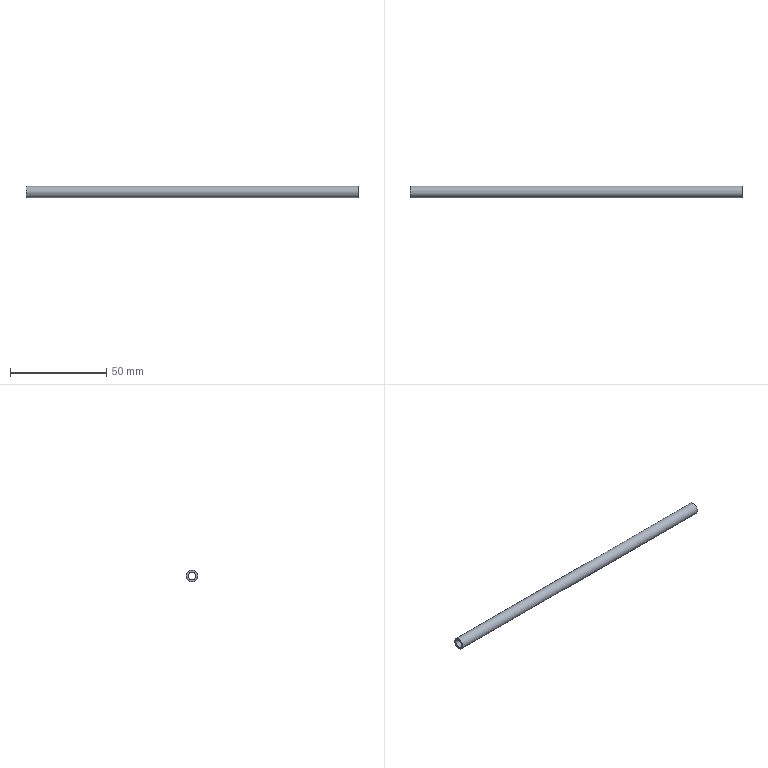Part | NX | features solid 2 | 1 solid | 4 faces | box 172.875 x 6 x 6 mm | volume 2716 mm3 | cylinder 2 | plane 2 | commonest cylinder face diameters 4 x1 6 x1
STEP:
#1=CARTESIAN_POINT('',(460.,-45.,347.));
#2=VERTEX_POINT('',#1);
#3=CARTESIAN_POINT('',(460.,-43.,347.));
#4=DIRECTION('',(-1.,0.,0.));
#5=DIRECTION('',(0.,-1.,0.));
#6=AXIS2_PLACEMENT_3D('',#3,#4,#5);
#7=CIRCLE('',#6,2.);
#8=EDGE_CURVE('',#2,#2,#7,.T.);
#9=ORIENTED_EDGE('',*,*,#8,.F.);
#10=EDGE_LOOP('',(#9));
#11=FACE_BOUND('',#10,.T.);
#12=CARTESIAN_POINT('',(287.125,-45.,347.));
#13=VERTEX_POINT('',#12);
#14=CARTESIAN_POINT('',(287.125,-43.,347.));
#15=DIRECTION('',(-1.,0.,0.));
#16=DIRECTION('',(0.,-1.,0.));
#17=AXIS2_PLACEMENT_3D('',#14,#15,#16);
#18=CIRCLE('',#17,2.);
#19=EDGE_CURVE('',#13,#13,#18,.T.);
#20=ORIENTED_EDGE('',*,*,#19,.T.);
#21=EDGE_LOOP('',(#20));
#22=FACE_BOUND('',#21,.T.);
#23=CARTESIAN_POINT('',(166.176,-43.,347.));
#24=DIRECTION('',(1.,0.,0.));
#25=DIRECTION('',(0.,1.,0.));
#26=AXIS2_PLACEMENT_3D('',#23,#24,#25);
#27=CYLINDRICAL_SURFACE('',#26,2.);
#28=ADVANCED_FACE('',(#11,#22),#27,.F.);
#29=CARTESIAN_POINT('',(460.,-46.,347.));
#30=VERTEX_POINT('',#29);
#31=CARTESIAN_POINT('',(460.,-43.,347.));
#32=DIRECTION('',(-1.,0.,0.));
#33=DIRECTION('',(0.,-1.,0.));
#34=AXIS2_PLACEMENT_3D('',#31,#32,#33);
#35=CIRCLE('',#34,3.);
#36=EDGE_CURVE('',#30,#30,#35,.T.);
#37=ORIENTED_EDGE('',*,*,#36,.T.);
#38=EDGE_LOOP('',(#37));
#39=FACE_BOUND('',#38,.T.);
#40=CARTESIAN_POINT('',(287.125,-46.,347.));
#41=VERTEX_POINT('',#40);
#42=CARTESIAN_POINT('',(287.125,-43.,347.));
#43=DIRECTION('',(-1.,0.,0.));
#44=DIRECTION('',(0.,-1.,0.));
#45=AXIS2_PLACEMENT_3D('',#42,#43,#44);
#46=CIRCLE('',#45,3.);
#47=EDGE_CURVE('',#41,#41,#46,.T.);
#48=ORIENTED_EDGE('',*,*,#47,.F.);
#49=EDGE_LOOP('',(#48));
#50=FACE_BOUND('',#49,.T.);
#51=CARTESIAN_POINT('',(166.176,-43.,347.));
#52=DIRECTION('',(1.,0.,0.));
#53=DIRECTION('',(0.,1.,0.));
#54=AXIS2_PLACEMENT_3D('',#51,#52,#53);
#55=CYLINDRICAL_SURFACE('',#54,3.);
#56=ADVANCED_FACE('',(#39,#50),#55,.T.);
#57=ORIENTED_EDGE('',*,*,#8,.T.);
#58=EDGE_LOOP('',(#57));
#59=FACE_BOUND('',#58,.T.);
#60=ORIENTED_EDGE('',*,*,#36,.F.);
#61=EDGE_LOOP('',(#60));
#62=FACE_BOUND('',#61,.T.);
#63=CARTESIAN_POINT('',(460.,-43.,347.));
#64=DIRECTION('',(-1.,0.,0.));
#65=DIRECTION('',(0.,-1.,0.));
#66=AXIS2_PLACEMENT_3D('',#63,#64,#65);
#67=PLANE('',#66);
#68=ADVANCED_FACE('',(#59,#62),#67,.F.);
#69=ORIENTED_EDGE('',*,*,#19,.F.);
#70=EDGE_LOOP('',(#69));
#71=FACE_BOUND('',#70,.T.);
#72=ORIENTED_EDGE('',*,*,#47,.T.);
#73=EDGE_LOOP('',(#72));
#74=FACE_BOUND('',#73,.T.);
#75=CARTESIAN_POINT('',(287.125,87.83,185.));
#76=DIRECTION('',(-1.,0.,0.));
#77=DIRECTION('',(0.,-1.,0.));
#78=AXIS2_PLACEMENT_3D('',#75,#76,#77);
#79=PLANE('',#78);
#80=ADVANCED_FACE('',(#71,#74),#79,.T.);
#81=CLOSED_SHELL('',(#28,#56,#68,#80));
#82=MANIFOLD_SOLID_BREP('',#81);
#83=(LENGTH_UNIT()NAMED_UNIT(*)SI_UNIT(.MILLI.,.METRE.));
#84=UNCERTAINTY_MEASURE_WITH_UNIT(LENGTH_MEASURE(0.00001),#83,'','');
#85=(NAMED_UNIT(*)PLANE_ANGLE_UNIT()SI_UNIT($,.RADIAN.));
#86=(NAMED_UNIT(*)SI_UNIT($,.STERADIAN.)SOLID_ANGLE_UNIT());
#87=(GEOMETRIC_REPRESENTATION_CONTEXT(3)GLOBAL_UNCERTAINTY_ASSIGNED_CONTEXT((#84))GLOBAL_UNIT_ASSIGNED_CONTEXT((#83,#85,#86))REPRESENTATION_CONTEXT('',''));
#88=ADVANCED_BREP_SHAPE_REPRESENTATION('',(#82),#87);